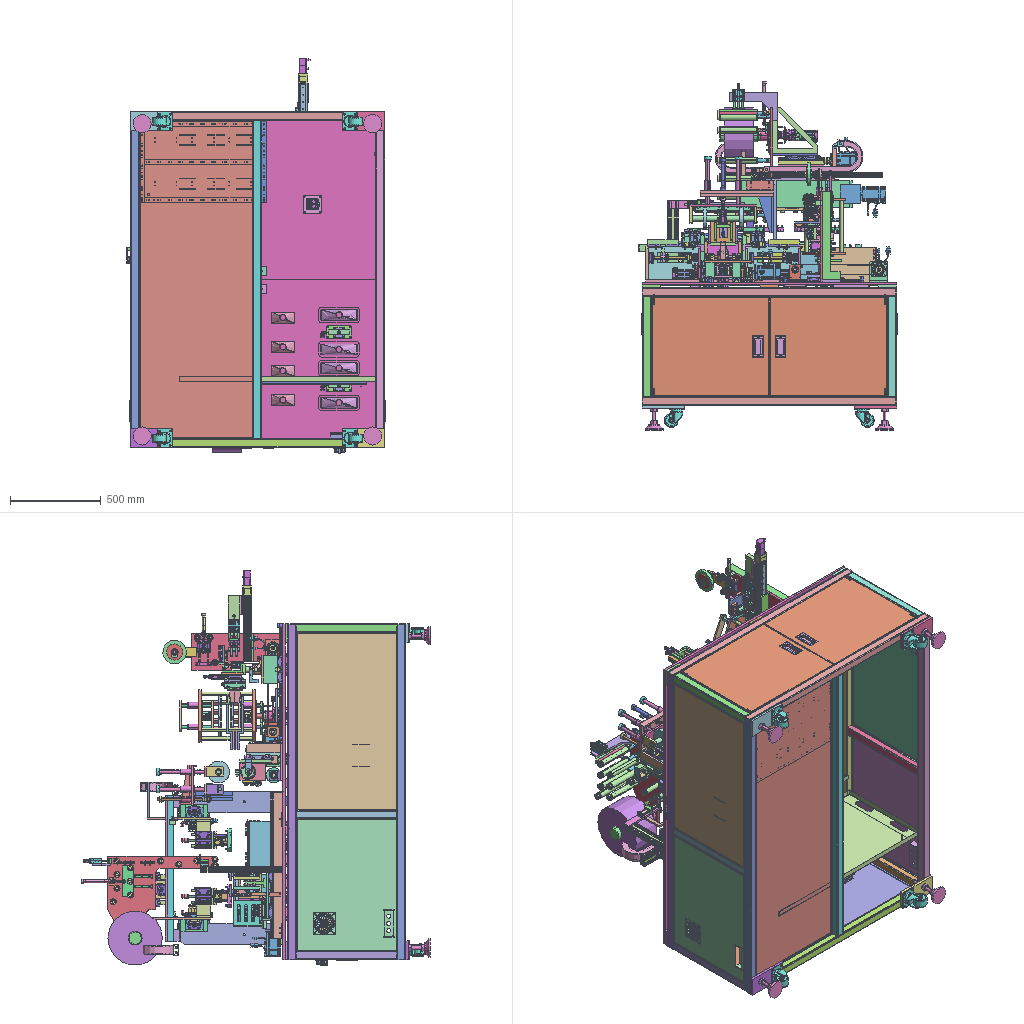Assembly | SolidWorks | 434 different items | 1246 placed | box 1425 x 1922 x 2174 mm
Parts list (item | name | quantity | parent item | size | volume | features), first 296 of 434 items:
1 | (subassembly) | x1 | - | - | 4869772 mm3 | features CompositeCurve 1
2 | (subassembly) | x3 | in 1 | 36 x 36 x 90 mm | 32561 mm3 | -
3 | (subassembly) | x2 | - | 274 x 476.237 x 327 mm | 5964747 mm3 | -
4 | (subassembly) | x2 | - | 273 x 282 x 303 mm | 1781179 mm3 | features InContextFeatHolder 4
5 | (subassembly) | x1 | - | - | - | -
6 | (subassembly) | x9 | in 5 | 34 x 292 x 34 mm | 157895 mm3 | -
7 | (subassembly) | x3 | in 5 | 34 x 267 x 34 mm | 150041 mm3 | -
8 | (subassembly) | x1 | in 5 | - | 5456068 mm3 | -
9 | (subassembly) | x1 | in 21 | - | 62540138 mm3 | -
10 | (subassembly) | x1 | - | 463.5 x 247.5 x 400.75 mm | 4348981 mm3 | features MirrorCompFeat 1
11 | (subassembly) | x1 | - | - | 21572641 mm3 | features CompositeCurve 32, InContextFeatHolder 3
12 | (subassembly) | x1 | - | 250 x 458 x 100.154 mm | 518648 mm3 | -
13 | (subassembly) | x1 | in 21 | 250.3 x 70.4 x 187 mm | 621495 mm3 | features AEMSimFeature 1
14 | (subassembly) | x1 | in 9 | - | 51712509 mm3 | -
15 | (subassembly) | x1 | - | - | 62540138 mm3 | features InContextFeatHolder 2
16 | (subassembly) | x10 | in 11, 21, 22 | 146.05 x 68.7 x 173.94 mm | 268514 mm3 | features ReferencePattern 3, AEMSimFeature 1, LocalLPattern 1
17 | (subassembly) | x1 | in 9 | 480 x 600 x 177.209 mm | 8711349 mm3 | -
18 | (subassembly) | x1 | - | - | 6443563 mm3 | features InContextFeatHolder 2, MirrorCompFeat 2
19 | (subassembly) | x2 | in 21 | 125.5 x 125.5 x 54.4 mm | 343156 mm3 | -
20 | (subassembly) | x1 | - | - | 6443563 mm3 | features InContextFeatHolder 8, MirrorCompFeat 2
21 | (subassembly) | x1 | - | - | - | features MirrorCompFeat 5, CompositeCurve 1
22 | (subassembly) | x1 | - | - | - | features InContextFeatHolder 8, CompositeCurve 2
23 | (subassembly) | x2 | in 22 | 148 x 205.5 x 218 mm | 1082273 mm3 | -
24 | (subassembly) | x1 | - | - | 10593540 mm3 | features CompositeCurve 3, InContextFeatHolder 2
25 | (subassembly) | x1 | - | - | - | features CompositeCurve 2, InContextFeatHolder 2
26 | (subassembly) | x1 | - | - | - | features CompositeCurve 3
27 | - | x3 | in 21 | 647 x 568 x 15 mm | 618702 mm3 | features ICE 5, FlatPattern 1, Helix 1, MirrorPattern 1, SMBaseFlange 1, SMMiteredFlange 1, SheetMetal 1, Sweep 1
28 | - | x1 | in 26 | 164 x 90 x 12 mm | 100831 mm3 | features Chamfer 1, Extrusion 1, Fillet 1
29 | - | x8 | in 26 | 40 x 30 x 12 mm | 14400 mm3 | features Extrusion 1
30 | - | x2 | in 26 | 180 x 150 x 10 mm | 230000 mm3 | features Extrusion 1, ICE 1, MirrorPattern 1
31 | - | x2 | in 26 | 180 x 150 x 6 mm | 138000 mm3 | features Extrusion 1, ICE 1, MirrorPattern 1
32 | - | x4 | in 26 | 12 x 12 x 75 mm | 8482 mm3 | features Extrusion 1
33 | - | x2 | in 26 | 60 x 90 x 14 mm | 56400 mm3 | features 3DProfileFeature 1, Chamfer 1, Extrusion 1, HoleWzd 1, ICE 1
34 | - | x1 | in 26 | 48 x 112.5 x 100 mm | 90182 mm3 | features Chamfer 1, Extrusion 1, ICE 1
35 | - | x1 | in 26 | 43 x 28 x 20 mm | 2700 mm3 | features FlatPattern 1, SMBaseFlange 1, SheetMetal 1
36 | - | x1 | in 26 | 95.861 x 40 x 61 mm | 9071 mm3 | features ICE 3, Extrusion 1
37 | - | x1 | in 1 | 17 x 58 x 27 mm | 21446 mm3 | features ICE 3, 3DProfileFeature 1, Extrusion 1, Fillet 1, HoleWzd 1
38 | - | x1 | in 21 | 647 x 568 x 78 mm | 637931 mm3 | features ICE 6, Cut 2, MirrorPattern 2, BossThin 1, Fillet 1, FlatPattern 1, Helix 1, SMBaseFlange 1, SMMiteredFlange 1, SheetMetal 1, Sweep 1, WeldmentFeature 1
39 | - | x1 | in 1 | 18 x 27 x 4 mm | 1881 mm3 | features Extrusion 1, ICE 1, LPattern 1, MirrorPattern 1
40 | - | x2 | in 1 | 10 x 27 x 4 mm | 1033 mm3 | features Extrusion 1, ICE 1, LPattern 1, MirrorPattern 1
41 | - | x2 | in 1 | 80 x 37 x 8 mm | 8818 mm3 | features ICE 4, 3DProfileFeature 1, Chamfer 1, Extrusion 1, Fillet 1, HoleWzd 1, MirrorPattern 1
42 | - | x2 | in 1 | 4 x 4 x 37 mm | 464.956 mm3 | features Extrusion 1
43 | - | x2 | in 1 | 9 x 9 x 28.5 mm | 1584 mm3 | features Extrusion 1
44 | - | x2 | in 1 | 4 x 4 x 47 mm | 590.619 mm3 | features Extrusion 1
45 | - | x1 | in 1 | 47 x 62 x 36 mm | 37251 mm3 | features ICE 6, 3DProfileFeature 2, HoleWzd 2, Extrusion 1, Fillet 1
46 | - | x1 | in 1 | 8 x 8 x 55 mm | 2765 mm3 | features Extrusion 1
47 | - | x2 | in 1 | 14 x 14 x 6 mm | 811.438 mm3 | features 3DProfileFeature 1, Chamfer 1, Extrusion 1, HoleWzd 1
48 | - | x1 | in 1 | 300 x 64 x 22.5 mm | 298859 mm3 | features ICE 4, Fillet 2, Extrusion 1, MirrorPattern 1
49 | - | x1 | in 21 | 1400 x 680 x 1850 mm | 13190709 mm3 | features WeldCornerFeat 8, Chamfer 4, HoleWzd 4, ICE 4, MirrorSolid 4, WeldMemberFeat 4, WeldmentFeature 1
50 | - | x1 | in 1 | 200 x 500 x 12 mm | 1093684 mm3 | features ICE 6, Fillet 2, Extrusion 1
51 | - | x1 | in 1 | 150 x 10 x 55 mm | 82500 mm3 | features Extrusion 1
52 | - | x1 | in 1 | 50 x 50 x 111 mm | 52677 mm3 | features ICE 3, Extrusion 1, RevCut 1
53 | - | x1 | in 1 | 46 x 40 x 46 mm | 14326 mm3 | features Revolution 1
54 | - | x1 | in 1 | 50 x 150 x 10 mm | 69893 mm3 | features Extrusion 1, ICE 1
55 | - | x1 | in 1 | 90 x 4 x 90 mm | 20564 mm3 | features Extrusion 1, ICE 1
56 | - | x1 | in 1 | 34 x 34 x 10 mm | 3614 mm3 | features Extrusion 1, HoleWzd 1
57 | - | x2 | in 1 | 87 x 22 x 12 mm | 17341 mm3 | features 3DProfileFeature 1, Extrusion 1, Fillet 1, HoleWzd 1, ICE 1, MirrorPattern 1
58 | - | x2 | in 1 | 8 x 8 x 140 mm | 7037 mm3 | features Extrusion 1
59 | - | x1 | in 1 | 25 x 72 x 50 mm | 71856 mm3 | features 3DProfileFeature 1, Chamfer 1, Extrusion 1, HoleWzd 1
60 | - | x1 | in 21 | 550 x 973 x 40 mm | 869590 mm3 | features ICE 2, BossThin 1, FlatPattern 1, SMBaseFlange 1, SMMiteredFlange 1, SheetMetal 1
61 | - | x1 | in 1 | 30 x 61 x 5 mm | 7526 mm3 | features Extrusion 1, Fillet 1
62 | - | x1 | in 1 | 53 x 14 x 63.5 mm | 9599 mm3 | features ICE 2, Extrusion 1
63 | - | x3 | in 2 | 12 x 12 x 90 mm | 9933 mm3 | features 3DProfileFeature 3, Extrusion 1, HoleWzd 1, ICE 1, LPattern 1, LibraryFeature 1, RefAxis 1, RevCut 1
64 | - | x4 | in 1, 2 | 27 x 27 x 50 mm | 13441 mm3 | features MirrorPattern 2, Extrusion 1, ICE 1, LPattern 1, RevCut 1
65 | - | x1 | in 1 | 90 x 4 x 90 mm | 23241 mm3 | features Extrusion 1, ICE 1
66 | - | x1 | in 1 | 45 x 57 x 10 mm | 13030 mm3 | features Extrusion 1, Fillet 1, ICE 1
67 | - | x1 | in 1 | 65 x 76 x 12 mm | 50562 mm3 | features ICE 2, 3DProfileFeature 1, Extrusion 1, HoleWzd 1
68 | - | x1 | in 1 | 80 x 60 x 12 mm | 45558 mm3 | features ICE 2, Extrusion 1, Fillet 1
69 | - | x1 | in 1 | 36 x 43 x 12 mm | 15546 mm3 | features ICE 3, Extrusion 1
70 | - | x2 | in 1 | 17.5 x 29 x 18 mm | 4245 mm3 | features ICE 3, Chamfer 1, Extrusion 1
71 | - | x2 | in 21 | 1400 x 925 x 14 mm | 18130000 mm3 | features Extrusion 1
72 | - | x1 | in 1 | 40 x 74.5 x 20 mm | 23378 mm3 | features ICE 2, Extrusion 1, LPattern 1
73 | - | x1 | in 1 | 44 x 35 x 13 mm | 17580 mm3 | features ICE 2, Extrusion 1, LPattern 1, MirrorPattern 1
74 | - | x1 | in 1 | 140 x 34 x 90 mm | 116009 mm3 | features ICE 2, Extrusion 1
75 | - | x2 | in 1, 10 | 43 x 22 x 0.4 mm | 344.471 mm3 | features Extrusion 1, ICE 1
76 | - | x1 | in 1 | 120 x 15 x 22 mm | 24706 mm3 | features ICE 4, Extrusion 1
77 | - | x1 | in 1 | 60 x 15 x 3 mm | 2658 mm3 | features 3DProfileFeature 1, Extrusion 1, HoleWzd 1
78 | - | x1 | in 1 | 55 x 100 x 12 mm | 58500 mm3 | features Extrusion 1, ICE 1
79 | - | x1 | in 1 | 200 x 100 x 12 mm | 240000 mm3 | features Extrusion 1
80 | - | x2 | in 1 | 98 x 488 x 12 mm | 292248 mm3 | features Chamfer 1, Extrusion 1, Fillet 1, ICE 1
81 | - | x8 | in 1, 2 | 36 x 36 x 8 mm | 3457 mm3 | features Extrusion 1, HoleWzd 1
82 | - | x1 | in 22 | 270 x 14 x 440 mm | 1620625 mm3 | features ICE 3, 3DProfileFeature 1, Extrusion 1, HoleWzd 1
83 | - | x6 | in 3 | 25 x 25 x 170 mm | 38250 mm3 | features Extrusion 1
84 | - | x2 | in 3 | 25 x 13 x 170 mm | 27963 mm3 | features 3DProfileFeature 1, Extrusion 1, HoleWzd 1
85 | - | x2 | in 3 | 130 x 12 x 180 mm | 252000 mm3 | features Extrusion 1
86 | - | x2 | in 3 | 210 x 12 x 260 mm | 560402 mm3 | features Chamfer 2, MirrorPattern 2, 3DProfileFeature 1, Extrusion 1, HoleWzd 1, ICE 1, LPattern 1
87 | - | x4 | in 3 | 23 x 23 x 180 mm | 21634 mm3 | features ICE 2, Extrusion 1, MirrorPattern 1
88 | - | x4 | in 3 | 160 x 25 x 7 mm | 28000 mm3 | features Extrusion 1
89 | - | x2 | in 3 | 140 x 25 x 5 mm | 17500 mm3 | features Extrusion 1
90 | - | x4 | in 3 | 16 x 22.5 x 190 mm | 52215 mm3 | features Chamfer 2, Extrusion 1, ICE 1
91 | - | x2 | in 3 | 18 x 16 x 190 mm | 52178 mm3 | features Chamfer 1, Extrusion 1, ICE 1
92 | - | x2 | in 3 | 135 x 70 x 8 mm | 55222 mm3 | features ICE 3, Chamfer 1, Extrusion 1
93 | - | x1 | in 22 | 55 x 44 x 35 mm | 54034 mm3 | features HoleWzd 2, 3DProfileFeature 1, Extrusion 1
94 | - | x4 | in 3 | 16 x 16 x 280 mm | 56297 mm3 | features Extrusion 1
95 | - | x2 | in 3 | 60 x 10 x 120 mm | 62330 mm3 | features ICE 2, Chamfer 1, Extrusion 1
96 | - | x8 | in 3 | 12 x 12 x 40 mm | 4146 mm3 | features 3DProfileFeature 1, Extrusion 1, HoleWzd 1, MirrorPattern 1
97 | - | x2 | in 3 | 25 x 10 x 120 mm | 26926 mm3 | features ICE 2, Extrusion 1
98 | - | x2 | in 3 | 19 x 18 x 7 mm | 1848 mm3 | features Extrusion 1
99 | - | x8 | in 3 | 24 x 24 x 10 mm | 2386 mm3 | features Extrusion 1
100 | - | x4 | in 3 | 260 x 15 x 5 mm | 19460 mm3 | features Chamfer 1, Extrusion 1
101 | - | x2 | in 3 | 41.958 x 24 x 12 mm | 3447 mm3 | features Extrusion 1, ICE 1
102 | - | x2 | in 3 | 260 x 20 x 20 mm | 43442 mm3 | features WeldMemberFeat 1, WeldmentFeature 1
103 | - | x2 | in 3 | 309 x 192.237 x 274 mm | 268790 mm3 | features EdgeFlange 2, FlatPattern 1, ICE 1, MirrorPattern 1, SMBaseFlange 1, SheetMetal 1
104 | - | x2 | in 22 | 25 x 53 x 800 mm | 1009600 mm3 | features Extrusion 1
105 | - | x2 | in 3 | 170 x 14 x 10 mm | 23403 mm3 | features 3DProfileFeature 1, Extrusion 1, HoleWzd 1, MirrorPattern 1
106 | - | x2 | in 3 | 248 x 185 x 6 mm | 275280 mm3 | features Extrusion 1
107 | - | x4 | in 3 | 224 x 84 x 115 mm | 101490 mm3 | features ICE 2, Blend 1, Extrusion 1, Shell 1
108 | - | x8 | in 3 | 40 x 30 x 12 mm | 6087 mm3 | features Extrusion 1, ICE 1, LPattern 1, MirrorPattern 1
109 | - | x8 | in 3 | 30 x 65 x 3 mm | 4682 mm3 | features Extrusion 1, ICE 1, MirrorPattern 1
110 | - | x4 | in 3 | 21 x 25 x 5 mm | 1150 mm3 | features Extrusion 1
111 | - | x2 | in 4 | 170 x 10 x 210 mm | 352545 mm3 | features MirrorPattern 2, Chamfer 1, Cut 1, Extrusion 1, ICE 1
112 | - | x8 | in 4 | 46 x 30 x 10 mm | 11809 mm3 | features 3DProfileFeature 1, Extrusion 1, HoleWzd 1, ICE 1, MirrorPattern 1
113 | - | x2 | in 4 | 135 x 180 x 8 mm | 157363 mm3 | features ICE 2, Chamfer 1, Extrusion 1
114 | - | x6 | in 4 | 80 x 42 x 10 mm | 29577 mm3 | features ICE 2, Chamfer 1, Extrusion 1, MirrorPattern 1
115 | - | x1 | in 22 | 48 x 93 x 100 mm | 106256 mm3 | features Chamfer 1, Extrusion 1
116 | - | x2 | in 4 | 58 x 62 x 10 mm | 30557 mm3 | features ICE 2, Chamfer 1, Extrusion 1, MirrorPattern 1
117 | - | x8 | in 4 | 20 x 20 x 150 mm | 47124 mm3 | features Extrusion 1
118 | - | x2 | in 4 | 245 x 10 x 210 mm | 367454 mm3 | features MirrorPattern 3, 3DProfileFeature 1, Chamfer 1, Cut 1, Extrusion 1, HoleWzd 1, ICE 1
119 | - | x4 | in 4 | 154 x 84 x 100 mm | 51797 mm3 | features ICE 2, Blend 1, Extrusion 1, Shell 1
120 | - | x2 | in 4 | 273 x 181.2 x 303 mm | 301154 mm3 | features Chamfer 1, ExtruThin 1, ICE 1
121 | - | x2 | in 11 | 600 x 150 x 14 mm | 1207472 mm3 | features ICE 3, Extrusion 1, Fillet 1
122 | - | x4 | in 11 | 25 x 33 x 600 mm | 457200 mm3 | features Extrusion 1
123 | - | x4 | in 11 | 14 x 550 x 115 mm | 786870 mm3 | features ICE 2, Chamfer 1, Extrusion 1
124 | - | x2 | in 11 | 300 x 12 x 115 mm | 414000 mm3 | features Extrusion 1
125 | - | x8 | in 11 | 74 x 74 x 20 mm | 33836 mm3 | features 3DProfileFeature 2, Chamfer 2, HoleWzd 2, Extrusion 1, Fillet 1
126 | - | x1 | in 22 | 25 x 90 x 24.5 mm | 55125 mm3 | features Extrusion 1
127 | - | x2 | in 11 | 272 x 25 x 25 mm | 133518 mm3 | features Extrusion 1
128 | - | x2 | in 11 | 300 x 180 x 12 mm | 604823 mm3 | features ICE 3, Extrusion 1, MirrorPattern 1
129 | - | x2 | in 11 | 112 x 95 x 100 mm | 206190 mm3 | features ICE 2, Chamfer 1, Extrusion 1
130 | - | x4 | in 11 | 34 x 80 x 162 mm | 152640 mm3 | features Extrusion 1, ICE 1, MirrorPattern 1
131 | - | x2 | in 11 | 145 x 125 x 20 mm | 332455 mm3 | features ICE 4, Chamfer 1, Extrusion 1
132 | - | x2 | in 11 | 91 x 80 x 38 mm | 128587 mm3 | features Extrusion 1, Fillet 1, ICE 1
133 | - | x2 | in 11 | 145 x 125 x 20 mm | 303441 mm3 | features ICE 6, Chamfer 1, Extrusion 1
134 | - | x4 | in 11 | 38 x 80 x 24 mm | 29184 mm3 | features Extrusion 1, ICE 1
135 | - | x1 | in 11 | 55 x 47 x 35 mm | 59809 mm3 | features HoleWzd 2, 3DProfileFeature 1, Extrusion 1
136 | - | x2 | in 11 | 18 x 8 x 30 mm | 2093 mm3 | features 3DProfileFeature 1, Extrusion 1, HoleWzd 1, ICE 1, MirrorPattern 1
137 | - | x1 | in 17 | 440 x 300 x 58 mm | 6630448 mm3 | features ICE 7, Fillet 2, Chamfer 1, Extrusion 1, HoleWzd 1, LPattern 1
138 | - | x1 | in 22 | 20 x 90 x 24.5 mm | 44100 mm3 | features Extrusion 1
139 | - | x6 | in 11 | 25 x 70 x 14 mm | 24500 mm3 | features Extrusion 1
140 | - | x2 | in 11 | 600 x 30 x 60 mm | 465086 mm3 | features WeldMemberFeat 1, WeldmentFeature 1
141 | - | x2 | in 11 | 170 x 214 x 10 mm | 60475 mm3 | features ICE 2, Chamfer 1, Extrusion 1, Fillet 1
142 | - | x2 | in 11 | 20 x 195 x 10 mm | 39000 mm3 | features Extrusion 1
143 | - | x2 | in 11 | 300 x 73 x 62 mm | 429281 mm3 | features ICE 6, Extrusion 1, Fillet 1
144 | - | x1 | in 5 | 600 x 515 x 14 mm | 1803753 mm3 | features ICE 11, Chamfer 4, Fillet 3, Cut 1, Extrusion 1
145 | - | x1 | in 5 | 30 x 30 x 17 mm | 3335 mm3 | features Extrusion 1
146 | - | x1 | in 5 | 65 x 68 x 120 mm | 106942 mm3 | features ICE 5, MirrorPattern 3, Chamfer 1, WeldMemberFeat 1, WeldmentFeature 1
147 | - | x1 | in 5 | 12 x 45 x 10 mm | 4126 mm3 | features 3DProfileFeature 1, Chamfer 1, Extrusion 1, HoleWzd 1, ICE 1, MirrorPattern 1
148 | - | x13 | in 6, 7, 10 | 210 x 34 x 34 mm | 85831 mm3 | features Revolution 1
149 | - | x1 | in 22 | 180 x 182 x 14 mm | 257706 mm3 | features ICE 5, Extrusion 1, Fillet 1
150 | - | x9 | in 6 | 20 x 20 x 275 mm | 57016 mm3 | features ICE 2, 3DProfileFeature 1, Extrusion 1, HoleWzd 1
151 | - | x12 | in 6, 7 | 33 x 33 x 14 mm | 9032 mm3 | features ICE 2, Chamfer 1, Extrusion 1
152 | - | x1 | in 5 | 170 x 60 x 12 mm | 111868 mm3 | features ICE 2, 3DProfileFeature 1, Extrusion 1, HoleWzd 1
153 | - | x1 | in 5 | 23 x 42 x 40 mm | 17172 mm3 | features Extrusion 1, ICE 1
154 | - | x1 | in 5 | 269 x 155 x 12 mm | 212510 mm3 | features Cut 1, Extrusion 1
155 | - | x1 | in 5 | 210 x 28 x 14 mm | 79716 mm3 | features Extrusion 1, ICE 1
156 | - | x1 | in 5 | 28 x 17 x 210 mm | 85260 mm3 | features Extrusion 1
157 | - | x1 | in 8 | 215 x 14 x 250 mm | 709650 mm3 | features ICE 2, Chamfer 1, Extrusion 1, Fillet 1
158 | - | x2 | in 8 | 250 x 245 x 12 mm | 232707 mm3 | features Extrusion 1
159 | - | x2 | in 8 | 25 x 28.5 x 250 mm | 162375 mm3 | features Extrusion 1
160 | - | x1 | in 22 | 55 x 75.5 x 30 mm | 98100 mm3 | features HoleWzd 2, 3DProfileFeature 1, Extrusion 1
161 | - | x1 | in 8 | 55 x 44 x 35 mm | 59279 mm3 | features HoleWzd 2, 3DProfileFeature 1, Extrusion 1
162 | - | x1 | in 8 | 250 x 800 x 14 mm | 1757091 mm3 | features ICE 2, Extrusion 1, Fillet 1
163 | - | x2 | in 8 | 800 x 14 x 30 mm | 336000 mm3 | features Extrusion 1
164 | - | x1 | in 8 | 45 x 101 x 100 mm | 97106 mm3 | features 3DProfileFeature 1, Chamfer 1, Extrusion 1, HoleWzd 1, ICE 1
165 | - | x3 | in 7 | 20 x 20 x 250 mm | 49162 mm3 | features ICE 2, 3DProfileFeature 1, Extrusion 1, HoleWzd 1
166 | - | x1 | in 14 | 1840 x 1100 x 1390 mm | 30476002 mm3 | features ICE 16, WeldCornerFeat 14, HoleWzd 8, WeldMemberFeat 7, MirrorPattern 3, Fillet 2, 3DProfileFeature 1, Cut 1, WeldmentFeature 1
167 | - | x1 | in 10 | 403 x 225.5 x 32 mm | 1138849 mm3 | features ICE 3, MoveFace 2, Extrusion 1
168 | - | x1 | in 10 | 240 x 25 x 12 mm | 71196 mm3 | features Extrusion 1, ICE 1
169 | - | x2 | in 10 | 23 x 31 x 10 mm | 4928 mm3 | features 3DProfileFeature 3, HoleWzd 3, ICE 2, Chamfer 1, Extrusion 1
170 | - | x2 | in 10 | 22 x 22 x 5 mm | 831.54 mm3 | features Extrusion 1
171 | - | x1 | in 22 | 60 x 180 x 14 mm | 46123 mm3 | features Extrusion 1, Fillet 1, ICE 1
172 | - | x2 | in 10 | 55 x 35 x 4 mm | 5554 mm3 | features Chamfer 1, Extrusion 1, ICE 1, MirrorPattern 1
173 | - | x1 | in 10 | 365 x 55 x 12 mm | 237663 mm3 | features ICE 2, Extrusion 1
174 | - | x2 | in 10 | 55 x 80 x 12 mm | 48578 mm3 | features ICE 3, 3DProfileFeature 1, Chamfer 1, Extrusion 1, HoleWzd 1
175 | - | x1 | in 10 | 20 x 14 x 370 mm | 68901 mm3 | features ICE 2, Extrusion 1
176 | - | x1 | in 10 | 32 x 30 x 63 mm | 43546 mm3 | features ICE 2, 3DProfileFeature 1, Extrusion 1, HoleWzd 1
177 | - | x2 | in 10 | 35 x 9 x 3 mm | 849.574 mm3 | features Extrusion 1
178 | - | x1 | in 10 | 50 x 12 x 3 mm | 1705 mm3 | features Extrusion 1
179 | - | x1 | in 10 | 365 x 55 x 12 mm | 237663 mm3 | features ICE 2, Extrusion 1
180 | - | x2 | in 10 | 55 x 94.5 x 12 mm | 49827 mm3 | features ICE 4, Chamfer 1, Extrusion 1
181 | - | x1 | in 10 | 30 x 30 x 361 mm | 247322 mm3 | features Extrusion 1, ICE 1, MirrorPattern 1
182 | - | x1 | in 22 | 150 x 14 x 200 mm | 400905 mm3 | features ICE 2, 3DProfileFeature 1, Extrusion 1, HoleWzd 1
183 | - | x1 | - | 217.5 x 60 x 150 mm | 433717 mm3 | features ICE 2, Chamfer 1, Extrusion 1, Fillet 1, MirrorPattern 1
184 | - | x1 | - | 217.5 x 90 x 50 mm | 220780 mm3 | features Chamfer 1, Extrusion 1, ICE 1
185 | - | x1 | in 12 | 30 x 450 x 60 mm | 348814 mm3 | features WeldMemberFeat 1, WeldmentFeature 1
186 | - | x1 | in 12 | 250 x 40 x 10 mm | 95200 mm3 | features Extrusion 1, ICE 1
187 | - | x2 | in 12 | 40 x 12 x 23 mm | 9230 mm3 | features ICE 5, Extrusion 1
188 | - | x1 | in 12 | 12 x 12 x 157 mm | 15432 mm3 | features ICE 2, Extrusion 1
189 | - | x2 | in 12 | 8 x 8 x 144 mm | 7238 mm3 | features Extrusion 1
190 | - | x1 | in 12 | 40 x 20 x 25 mm | 16355 mm3 | features ICE 5, 3DProfileFeature 1, Extrusion 1, HoleWzd 1
191 | - | x1 | in 12 | 70 x 55 x 4 mm | 7768 mm3 | features Fillet 2, ICE 2, Extrusion 1
192 | - | x7 | in 5, 22, 24, 25, 26 | - | 141786 mm3 | features BaseBody 32
193 | - | x1 | in 22 | 200 x 14 x 165 mm | 371300 mm3 | features Extrusion 1, Fillet 1, ICE 1
194 | - | x20 | in 16 | 22 x 64 x 22 mm | 21333 mm3 | features BaseBody 1
195 | - | x38 | in 3, 5, 11, 22, 24, 25, 26 | 13.7 x 28.4 x 26 mm | 1939 mm3 | features BaseBody 1
196 | - | x2 | in 13 | 21 x 8.5 x 8.5 mm | 552.853 mm3 | features BaseBody 1
197 | - | x1 | in 13 | 68.8 x 64 x 160 mm | 171745 mm3 | features BaseBody 2
198 | - | x1 | in 13 | 68.8 x 64 x 171.6 mm | 182520 mm3 | features BaseBody 1
199 | - | x2 | in 13 | 33 x 49.1 x 93 mm | 35639 mm3 | features BaseBody 1
200 | - | x2 | in 13 | 11.9 x 33 x 25 mm | 6485 mm3 | features BaseBody 1
201 | - | x1 | in 13 | 68.8 x 68.4 x 103.9 mm | 177481 mm3 | features BaseBody 5
202 | - | x1 | in 24 | 60 x 95 x 137 mm | 414579 mm3 | features BaseBody 8
203 | - | x1 | in 21 | 450 x 700 x 6 mm | 1886062 mm3 | features HoleWzd 2, Cut 1, Extrusion 1
204 | - | x3 | in 22 | 135 x 150 x 14 mm | 55621 mm3 | features Extrusion 1, Fillet 1, ICE 1
205 | - | x1 | in 14 | 150 x 3 x 150 mm | 65828 mm3 | features Extrusion 1, Fillet 1, HoleWzd 1, ICE 1
206 | - | x1 | in 17 | 480 x 600 x 153 mm | 803618 mm3 | features ICE 7, EdgeFlange 3, Cut 1, FlatPattern 1, SMBaseFlange 1, SheetMetal 1
207 | - | x1 | in 9 | 480 x 195.932 x 160.122 mm | 336686 mm3 | features EdgeFlange 8, ICE 2, Fillet 1, FlatPattern 1, SMBaseFlange 1, SheetMetal 1
208 | - | x6 | in 9 | 49.2 x 40 x 8 mm | 11464 mm3 | features HoleWzd 2, ICE 2, Chamfer 1, Extrusion 1
209 | - | x2 | in 14 | 718 x 1016 x 28.7 mm | 4599989 mm3 | features MoveCopyBody 3, Stock 3, ICE 2, HoleWzd 1, WeldMemberFeat 1, WeldmentFeature 1
210 | - | x2 | in 14 | 588 x 1016 x 28.7 mm | 3776300 mm3 | features MoveCopyBody 3, Stock 3, ICE 2, HoleWzd 1, WeldMemberFeat 1, WeldmentFeature 1
211 | - | x2 | in 14 | 479 x 716 x 28.7 mm | 2209048 mm3 | features MoveCopyBody 3, Stock 3, ICE 2, HoleWzd 1, WeldMemberFeat 1, WeldmentFeature 1
212 | - | x10 | in 16 | 60 x 26.5 x 140 mm | 117754 mm3 | features 3DProfileFeature 3, HoleWzd 3, Cut 1, Extrusion 1, LPattern 1
213 | - | x40 | in 16 | 15.02 x 42.2 x 146.05 mm | 33782 mm3 | features Boss 25, Cut 6, RevCut 5, Revolution 2, Extrusion 1, ICE 1
214 | - | x2 | in 4 | 41.439 x 18 x 38.614 mm | 6724 mm3 | features Chamfer 1, Extrusion 1, Sweep 1
215 | - | x1 | in 22 | 93 x 62 x 40 mm | 39399 mm3 | features ICE 5, 3DProfileFeature 1, Extrusion 1, Fillet 1, HoleWzd 1
216 | - | x2 | in 11 | 24 x 27.713 x 90.43 mm | 14815 mm3 | features ICE 3, Chamfer 2, Extrusion 1, MirrorPattern 1, Sweep 1
217 | - | x4 | in 11 | 53.2 x 29.75 x 23 mm | 14418 mm3 | features ICE 8, Revolution 1
218 | - | x1 | in 17 | 212.35 x 146.35 x 53.56 mm | 1066070 mm3 | features ICE 16, Fillet 5, MirrorPattern 2, Extrusion 1, HoleWzd 1
219 | - | x6 | in 9 | 49.2 x 17.45 x 45.25 mm | 22167 mm3 | features ICE 16, Chamfer 3, Fillet 3, Extrusion 1
220 | - | x1 | in 9 | 330 x 19.5 x 178 mm | 879010 mm3 | features ICE 7, Fillet 4, LPattern 2, Extrusion 1
221 | - | x2 | in 1, 5 | 142 x 64.5 x 30.5 mm | 123936 mm3 | features BaseBody 5, MoveFace 1
222 | - | x2 | in 3 | 57 x 57 x 276 mm | 233690 mm3 | features ICE 6, Extrusion 1, Fillet 1, MoveFace 1
223 | - | x5 | in 11, 22, 24 | 45 x 53 x 34 mm | 37006 mm3 | features BaseBody 1
224 | - | x2 | in 3 | 130 x 150 x 180 mm | 3150000 mm3 | features Extrusion 1
225 | - | x3 | in 25 | 9 x 6 x 50 mm | 1608 mm3 | features Extrusion 1
226 | - | x1 | in 22 | 60 x 180 x 14 mm | 45584 mm3 | features Cut 1, Extrusion 1, Fillet 1, ICE 1
227 | - | x18 | in 5, 11, 22, 24, 25, 26 | 9 x 6 x 75 mm | 2412 mm3 | features Extrusion 1
228 | - | x1 | in 22 | 9 x 6 x 75 mm | 2412 mm3 | features Extrusion 1
229 | - | x1 | in 10 | 15 x 15 x 240 mm | 42412 mm3 | features Extrusion 1
230 | - | x2 | in 10 | 16 x 16 x 250 mm | 50265 mm3 | features Extrusion 1
231 | - | x4 | in 10 | 20 x 20 x 265 mm | 83252 mm3 | features Extrusion 1
232 | - | x4 | in 11 | 24.892 x 60.174 x 63.5 mm | 25312 mm3 | features BaseBody 8
233 | - | x2 | in 1 | 45 x 32 x 32 mm | 7447 mm3 | features BaseBody 1
234 | - | x3 | in 10 | 120 x 120 x 20 mm | 212058 mm3 | features Extrusion 1
235 | - | x1 | in 17 | 30 x 78.5 x 40 mm | 52539 mm3 | features Boss 3, Revolution 2, Cut 1, Fillet 1
236 | - | x4 | in 25, 26 | 35 x 6 x 42 mm | 6903 mm3 | features BaseBody 1
237 | - | x2 | in 23 | 46 x 119 x 100 mm | 191222 mm3 | features ICE 2, MirrorPattern 2, Extrusion 1
238 | - | x2 | in 1 | 92 x 46 x 17 mm | 51092 mm3 | features BaseBody 2, MoveFace 1
239 | - | x8 | in 4 | 68 x 42 x 17 mm | 36294 mm3 | features BaseBody 2, MoveFace 1
240 | - | x4 | in 11 | 176.5 x 93 x 42 mm | 329147 mm3 | features BaseBody 3, MoveFace 1
241 | - | x6 | in 8, 11, 22, 25, 26 | 104.241 x 167.272 x 173.3 mm | 816769 mm3 | features BaseBody 1
242 | - | x4 | in 3 | 17.5 x 17.5 x 55 mm | 1534 mm3 | features BaseBody 2, MoveFace 2, CoordSys 1
243 | - | x2 | in 25, 26 | 515 x 55 x 25 mm | 54325 mm3 | features ExtruThin 1
244 | - | x3 | in 22, 24 | 22 x 48 x 48 mm | 28934 mm3 | features BaseBody 1
245 | - | x1 | in 24 | 32 x 55 x 55 mm | 52760 mm3 | features BaseBody 1
246 | - | x2 | in 24 | 31 x 83 x 83 mm | 73230 mm3 | features MoveFace 2, BaseBody 1, ICE 1
247 | - | x2 | in 24 | 31 x 83 x 83 mm | 94794 mm3 | features MoveFace 2, BaseBody 1, ICE 1
248 | - | x1 | in 21 | 550 x 723 x 40 mm | 641172 mm3 | features ICE 3, BossThin 1, FlatPattern 1, SMBaseFlange 1, SMMiteredFlange 1, SheetMetal 1
249 | - | x2 | in 23 | 60 x 140 x 14 mm | 109393 mm3 | features ICE 2, Cut 1, Extrusion 1, Fillet 1, HoleWzd 1
250 | - | x3 | in 22, 24 | 34 x 45 x 45 mm | 28395 mm3 | features BaseBody 1
251 | - | x2 | in 5 | 32 x 48 x 48 mm | 32144 mm3 | features BaseBody 1
252 | - | x2 | in 25, 26 | 32 x 55 x 55 mm | 48801 mm3 | features BaseBody 1, ICE 1
253 | - | x3 | in 24, 25, 26 | 44 x 55 x 55 mm | 58825 mm3 | features BaseBody 1
254 | - | x1 | in 17 | 30 x 78.5 x 40 mm | 52539 mm3 | features Boss 3, Revolution 2, Cut 1, Fillet 1
255 | - | x2 | in 10 | 35 x 35 x 15 mm | 11416 mm3 | features Extrusion 1
256 | - | x4 | in 10 | 40 x 40 x 15 mm | 14137 mm3 | features Extrusion 1
257 | - | x7 | in 8, 11, 22, 24 | 38 x 43 x 60 mm | 55106 mm3 | features BaseBody 9
258 | - | x3 | in 8, 25, 26 | 10 x 56 x 10 mm | 1814 mm3 | features BaseBody 1, MoveFace 1
259 | - | x1 | in 10 | 214 x 25 x 22 mm | 42451 mm3 | features BaseBody 4, MoveFace 2
260 | - | x2 | in 23 | 45 x 102 x 18 mm | 31894 mm3 | features 3DProfileFeature 1, Extrusion 1, Fillet 1, HoleWzd 1, ICE 1, MirrorPattern 1
261 | - | x1 | in 5 | 318 x 25 x 22 mm | 45425 mm3 | -
262 | - | x4 | in 23 | 158 x 25 x 22 mm | 25129 mm3 | features BaseBody 4, MoveFace 2
263 | - | x1 | in 1 | 148 x 25 x 22 mm | 28789 mm3 | features BaseBody 4, MoveFace 2
264 | - | x2 | in 10 | 216 x 33 x 29 mm | 70074 mm3 | features BaseBody 4, MoveFace 2
265 | - | x20 | in 16 | 10 x 14.097 x 14.097 mm | 1197 mm3 | features Chamfer 1, Cut 1, Revolution 1
266 | - | x3 | in 24 | 18 x 45 x 18 mm | 5618 mm3 | features BaseBody 1, MoveFace 1
267 | - | x5 | in 1, 5, 23 | 10 x 43.5 x 10 mm | 1326 mm3 | features BaseBody 1, MoveFace 1
268 | - | x1 | in 17 | 30 x 78.5 x 40 mm | 52539 mm3 | features Boss 3, Revolution 2, Cut 1, Fillet 1
269 | - | x3 | in 24 | 17 x 8 x 19.63 mm | 1532 mm3 | features BaseBody 1
270 | - | x1 | in 9 | 100 x 455.5 x 100 mm | 698561 mm3 | features ICE 17, Fillet 6, BossThin 1, Chamfer 1, CirPattern 1, Extrusion 1, RefAxis 1, RevCut 1
271 | - | x4 | in 23 | 60 x 60 x 12 mm | 30812 mm3 | features 3DProfileFeature 1, Extrusion 1, HoleWzd 1, ICE 1, LPattern 1, MirrorPattern 1
272 | - | x4 | in 22 | 64.1 x 19.5 x 34 mm | 30819 mm3 | features BaseBody 1
273 | - | x35 | in 1, 8, 11, 22, 24, 25, 26 | 83.53 x 22 x 42 mm | 51004 mm3 | features BaseBody 1
274 | - | x10 | in 5, 23 | 42.1 x 12 x 32 mm | 11943 mm3 | features BaseBody 1
275 | - | x4 | in 3 | 14 x 20 x 7 mm | 1562 mm3 | features ICE 2, Extrusion 1, Fillet 1, MirrorPattern 1
276 | - | x1 | - | 120 x 60 x 15 mm | 20369 mm3 | features Boss 2, Cut 1, Extrusion 1, Fillet 1, Shell 1
277 | - | x1 | in 24 | 51 x 53 x 31 mm | 42368 mm3 | features BaseBody 2
278 | - | x4 | in 24 | 55 x 61 x 35 mm | 59445 mm3 | features BaseBody 2
279 | - | x2 | in 5, 26 | 86 x 98 x 98 mm | 237483 mm3 | features BaseBody 5
280 | - | x2 | in 1 | 11 x 11 x 12 mm | 96.988 mm3 | features Helix 1, ICE 1, Sweep 1
281 | - | x1 | in 1 | 30 x 30 x 40 mm | 1368 mm3 | features Helix 1, ICE 1, Sweep 1
282 | - | x4 | in 23 | 30 x 95 x 11 mm | 13468 mm3 | features ICE 2, Extrusion 1, Fillet 1
283 | - | x20 | in 16 | 15.2 x 36.1 x 31.083 mm | 5569 mm3 | features BaseBody 1
284 | - | x1 | in 17 | 40 x 67.009 x 40 mm | 39506 mm3 | features Cut 3, Fillet 3, Boss 2, Revolution 1
285 | - | x1 | in 24 | 32 x 45 x 45 mm | 40105 mm3 | features BaseBody 4
286 | - | x4 | in 3 | 20 x 36 x 106 mm | 20303 mm3 | features BaseBody 1
287 | - | x2 | in 11 | 572.2 x 175 x 53 mm | 617417 mm3 | features BaseBody 3
288 | - | x1 | in 25 | 480.2 x 175 x 53 mm | 549939 mm3 | features BaseBody 3
289 | - | x1 | in 13 | 28.083 x 33.4 x 14 mm | 4394 mm3 | features BaseBody 1
290 | - | x1 | in 25 | 47 x 11 x 47 mm | 10056 mm3 | features BaseBody 1
291 | - | x7 | in 8, 11, 22, 24 | 20 x 43 x 60 mm | 35576 mm3 | features BaseBody 3
292 | - | x1 | in 5 | 300 x 300 x 160 mm | 10583900 mm3 | features Extrusion 1
293 | - | x2 | in 23 | 60 x 140 x 14 mm | 109393 mm3 | features ICE 2, Cut 1, Extrusion 1, Fillet 1, HoleWzd 1
294 | - | x1 | in 25 | 165 x 67.1 x 26.6 mm | 85115 mm3 | features BaseBody 9, MoveFace 3
295 | - | x1 | in 10 | 336 x 61 x 36 mm | 312285 mm3 | features BaseBody 4, MoveFace 1
296 | - | x4 | in 21 | 105 x 104 x 107.5 mm | 293798 mm3 | features ICE 10, Fillet 8, Chamfer 1, Extrusion 1
Mates (type | each side: item.copy, entity, surface, feature), first 256 of 2087 lines:
In the top assembly
Coincident | 71.1 face plane  Boss - Extrude 1 | 104.1 face plane  Boss - Extrude 1
Parallel | 71.1 face plane  Boss - Extrude 1 | 104.1 edge
Coincident | 71.2 face plane  Boss - Extrude 1 | 374.1 face plane  Boss - Extrude 1
Width | 104.2 face plane  Boss - Extrude 1 | 104.1 face plane  Boss - Extrude 1 | 374.1 face plane  Boss - Extrude 1 | 374.1 face plane  Boss - Extrude 1
Coincident | 71.2 face plane  Boss - Extrude 1 | 322.1 face plane  Boss - Extrude 1
Width | 104.2 face plane  Boss - Extrude 1 | 104.1 face plane  Boss - Extrude 1 | 390.1 face plane  Boss - Extrude 1 | 390.1 face plane  Boss - Extrude 1
DistanceDim | 407.1 face plane  Boss - Extrude 1 | 374.1 face plane  Boss - Extrude 1
DistanceDim | 374.1 face plane  Boss - Extrude 1 | 104.2 face plane  Boss - Extrude 1
DistanceDim | 374.1 face plane  Boss - Extrude 1 | 71.2 face plane  Boss - Extrude 1
Coincident | 71.2 face plane  Boss - Extrude 1 | 322.2 face plane  Boss - Extrude 1
Parallel | 71.2 face plane  Boss - Extrude 1 | 322.3 face plane  Boss - Extrude 1
Coincident | 71.2 face plane  Boss - Extrude 1 | 79.1 face plane  Boss - Extrude 1
Coincident | 71.1 face plane  Boss - Extrude 1 | 103.1 face plane  Edge - Flange 2
Parallel | 71.1 face plane  Boss - Extrude 1 | 103.1 face plane  Base - Flange 1
Coincident | 71.1 face plane  Boss - Extrude 1 | 103.2 face plane  Edge - Flange 2
Coincident | 103.1 face plane  Base - Flange 1 | 103.2 face plane  Base - Flange 1
Coincident | 71.1 face plane  Boss - Extrude 1 | 120.1 face plane  Boss - Extrude 1
Width | 103.2 face plane  Base - Flange 1 | 103.2 face plane  Base - Flange 1 | 120.1 face plane  Extrude - Thin-Wall 1 | 120.1 face plane  Extrude - Thin-Wall 1
Coincident | 71.1 face plane  Boss - Extrude 1 | 120.2 face plane  Boss - Extrude 1
Coincident | 120.1 face plane  Extrude - Thin-Wall 1 | 120.2 face plane  Extrude - Thin-Wall 1
Width | 103.1 face plane  Base - Flange 1 | 103.1 face plane  Base - Flange 1 | 120.2 face plane  Extrude - Thin-Wall 1 | 120.2 face plane  Extrude - Thin-Wall 1
DistanceDim | 103.1 face plane  Base - Flange 1 | 103.2 face plane  Base - Flange 1
DistanceDim | 241.1 face plane  Import 1 | 71.1 face plane  Boss - Extrude 1
Coincident | 71.1 face plane  Boss - Extrude 1 | 124.1 face plane  Boss - Extrude 1
Parallel | 71.1 face plane  Boss - Extrude 1 | 124.1 face plane  Boss - Extrude 1
Parallel | 71.1 face plane  Boss - Extrude 1 | 162.1 face plane  Boss - Extrude 1
Parallel | 71.1 face plane  Boss - Extrude 1 | 163.1 face plane  Boss - Extrude 1
DistanceDim | 123.1 face plane  Boss - Extrude 1 | 104.2 face plane  Boss - Extrude 1
Coincident | assembly face | 162.1 face plane  Boss - Extrude 1 | 2 times
Coincident | assembly face | 163.1 face plane  Boss - Extrude 1
Coincident | 143.1 face plane  Boss - Extrude 2 | 163.1 face plane  Boss - Extrude 1
Coincident | 143.1 face plane  Boss - Extrude 3 | 162.1 face plane  Boss - Extrude 1
Coincident | 143.1 face plane  Boss - Extrude 1 | 162.1 face plane  Boss - Extrude 1
DistanceDim | 71.2 face plane  Boss - Extrude 1 | 79.1 face plane  Boss - Extrude 1
Parallel | 71.1 face plane  Boss - Extrude 1 | 167.1 face plane  Boss - Extrude 1
Width | 346.1 face plane _BFU41-6008ZZ-L801-001-1-solid1 | 346.1 face plane _BFU41-6008ZZ-L801-001-1-solid1 | 325.1 face plane  Import 1 | 325.1 face plane  Import 1
Coincident | 123.2 face plane  Boss - Extrude 1 | 167.1 face plane  Boss - Extrude 2
Coincident | 167.1 face plane  Boss - Extrude 1 | 183.1 face plane  Boss - Extrude 1 | 2 times
Coincident | 121.1 face plane  Boss - Extrude 1 | 183.1 face plane  Boss - Extrude 1
Coincident | 123.2 face plane  Boss - Extrude 1 | 183.1 face plane  Boss - Extrude 1
Coincident | 123.2 face plane  Boss - Extrude 1 | 184.1 face plane  Boss - Extrude 1 | 2 times
Coincident | 167.1 face plane  Boss - Extrude 1 | 184.1 face plane  Boss - Extrude 1
Coincident | 71.1 face plane  Boss - Extrude 1 | 185.1 face plane  Industrial Aluminium Profile 30 X 60G X R1.5(1)
In subassembly 24
Concentric | 366.1 face cylinder  Boss - Extrude 1 | 246.1 face cylinder  Cut - Extrude 1
Coincident | 366.1 face plane  Boss - Extrude 2 | 246.1 face plane  Import 1
Coincident | 367.1 face plane  Revolve 1 | 246.1 face plane  Import 1
DistanceDim | 333.1 face plane _CPHCK-D35-A15-B15_base_b-1-solid1 | 278.1 face plane _BGF01-6004ZZ-h35-N_AN_AE-1-solid1
Concentric | 317.1 face cylinder  Boss - Extrude 3 | 278.1 face cylinder _BAY6004ZZ-009-1-solid1
Coincident | 317.1 face plane  Boss - Extrude 1 | 278.1 face plane _BAY6004ZZ-009-1-solid1
Coincident | 278.2 face plane _BGF01-6004ZZ-h35-N_AN_AE-1-solid1 | 374.2 face plane  Boss - Extrude 1 | 3 times
Concentric | 300.1 face cylinder _MQR2-M5(0)_AP-1-solid1 | 364.1 face cylinder  Boss - Extrude 1
Coincident | 300.1 face plane _MQR2-M5(0)_AP-1-solid1 | 364.1 face plane  Boss - Extrude 1
Parallel | 362.1 face plane  Boss - Extrude 1 | 364.1 face plane  Boss - Extrude 1
Coincident | 273.1 face plane  Import 1 | 362.1 face plane  Boss - Extrude 1 | 2 times
Width | 362.1 face plane  Boss - Extrude 1 | 362.1 face plane  Boss - Extrude 1 | 365.1 face plane  Boss - Extrude 1 | 365.1 face plane  Boss - Extrude 1
Coincident | 362.1 face plane  Boss - Extrude 1 | 368.1 face plane  Boss - Extrude 1 | 2 times
Coincident | 362.1 face plane  Boss - Extrude 1 | 273.2 face plane  Import 1 | 2 times
Coincident | 362.1 face plane  Boss - Extrude 1 | 273.3 face plane  Import 1
Coincident | 273.1 face plane  Import 1 | 273.4 face plane  Import 1
Coincident | 322.4 face plane  Boss - Extrude 1 | 273.4 face plane  Import 1
Width | 273.4 face plane  Import 1 | 273.4 face plane  Import 1 | 322.4 face plane  Boss - Extrude 1 | 322.4 face plane  Boss - Extrude 1
Coincident | 361.1 face plane  Cut - Extrude 1 | 322.4 face plane  Boss - Extrude 1 | 2 times
Coincident | 361.1 face plane  Boss - Extrude 1 | 322.4 face plane  Boss - Extrude 1
Width | 322.4 face plane  Boss - Extrude 1 | 322.5 face plane  Boss - Extrude 1 | 257.1 face plane _TSPB-12_base-1-solid1 | 257.1 face plane _TSPB-12_base-1-solid1
Coincident | 322.4 edge | 273.3 face plane  Import 1
Concentric | 257.1 face cylinder _tspb_BNTA-M12-1-solid1 | 291.1 face cylinder _spbf_BCA-A10-D26-B8-1-solid1
Parallel | 361.1 face plane  Boss - Extrude 1 | 291.1 face plane _SPBF-12_base-1-solid1
Coincident | 291.1 face plane _spbf_BCA-A10-D26-B8-1-solid1 | 314.1 face plane  Import 1
Coincident | 361.1 face plane  Cut - Extrude 1 | 322.5 face plane  Boss - Extrude 1 | 2 times
Coincident | 361.1 face plane  Boss - Extrude 1 | 322.5 face plane  Boss - Extrude 1
Coincident | 361.1 face plane  Boss - Extrude 1 | 257.1 face plane _TSPB-12_base-1-solid1
Parallel | 361.1 face plane  Boss - Extrude 1 | 365.1 face plane  Boss - Extrude 1
Parallel | 361.1 face plane  Boss - Extrude 1 | 223.1 face plane  Import 1
Coincident | 361.1 face plane  Boss - Extrude 1 | 278.2 face plane _BGF01-6004ZZ-h35-N_AN_AE-1-solid1
Coincident | 322.5 face plane  Boss - Extrude 1 | 273.1 face plane  Import 1
Width | 273.1 face plane  Import 1 | 273.1 face plane  Import 1 | 322.5 face plane  Boss - Extrude 1 | 322.5 face plane  Boss - Extrude 1
Coincident | 322.5 face plane  Boss - Extrude 1 | 273.2 face plane  Import 1
Concentric | 257.1 face cylinder _TSPB-12_ring-2-solid1 | 314.1 face cylinder  Import 1
Coincident | 257.1 face plane _TSPB-12_ring-2-solid1 | 314.1 face plane  Import 1
Concentric | 314.1 face cylinder  Import 1 | 223.1 face cylinder  Import 1
Coincident | 300.1 face plane _MQR2-M5(0)_BODY-1-solid1 | 363.1 face plane  Boss - Extrude 1
Coincident | 247.1 face plane  Import 1 | 369.1 face plane  Boss - Extrude 1
Width | 247.1 face plane  Import 1 | 247.1 face plane  Import 1 | 285.1 face plane _LGA-W32-D45_pulley-1-solid1 | 285.1 face plane _LGA-W32-D45_pulley-1-solid1
Coincident | 368.1 face plane  Boss - Extrude 1 | 372.1 face plane  Boss - Extrude 1
DistanceDim | 372.1 face plane  Boss - Extrude 1 | 368.1 face plane  Boss - Extrude 1
Concentric | 372.1 face cylinder  Boss - Extrude 1 | 266.1 face cylinder  Import 1
Coincident | 372.1 face plane  Boss - Extrude 1 | 373.1 face plane  Boss - Extrude 1
Coincident | 372.1 edge | 269.1 face plane  Import 1
Coincident | 368.1 face plane  Boss - Extrude 1 | 371.1 face plane  Boss - Extrude 1 | 2 times
DistanceDim | 371.1 face plane  Boss - Extrude 1 | 368.1 face plane  Boss - Extrude 1
Concentric | 285.1 face cylinder _LGA_BCA-A12-D32-B10-2-solid1 | 266.1 face cylinder  Import 1
Coincident | 285.1 face plane _LGA_BCA-A12-D32-B10-2-solid1 | 266.1 face plane  Import 1
Concentric | 266.1 face cylinder  Import 1 | 373.1 face cylinder  Boss - Extrude 1
Concentric | 266.1 face cylinder  Import 1 | 269.1 face cylinder  Import 1
Coincident | 273.2 face plane  Import 1 | 273.3 face plane  Import 1
Concentric | 317.1 face cylinder  Boss - Extrude 4 | 333.1 face cylinder _CPHCK-D35-A15-B15_base_b-1-solid1
Width | 278.2 face plane _BGF01-6004ZZ-h35-N_AN_AE-1-solid1 | 278.2 face plane _BGF01-6004ZZ-h35-N_AN_AE-1-solid1 | 371.1 face plane  Boss - Extrude 1 | 371.1 face plane  Boss - Extrude 1
Concentric | 317.1 face cylinder  Boss - Extrude 2 | 278.2 face cylinder _BAY6004ZZ-009-1-solid1
Coincident | 317.1 edge | 278.2 face plane _BAY6004ZZ-009-1-solid1
Concentric | 223.1 face cylinder  Import 1 | 365.1 face cylinder  Boss - Extrude 1
Coincident | 223.1 face plane  Import 1 | 365.1 face plane  Boss - Extrude 1
Concentric | 318.1 face cylinder _BTL-22_base-1-solid1 | 371.1 face cylinder  Boss - Extrude 1
DistanceDim | 318.1 face plane _BTL-22_base-1-solid1 | 371.1 face plane  Boss - Extrude 1
Parallel | 318.1 plane | 371.1 face plane  Boss - Extrude 1
Tangent | 367.1 face plane  Revolve 1 | 318.1 face cylinder _BTL-22_base-1-solid1
Concentric | 338.1 face cylinder  Boss - Extrude 1 | 317.1 face cylinder  Boss - Extrude 1
Concentric | 338.1 face cylinder  Boss - Extrude 1 | 366.1 face cylinder  Boss - Extrude 1
Coincident | 338.1 face plane  Boss - Extrude 2 | 366.1 face plane  Boss - Extrude 2
Concentric | 366.1 face cylinder  Boss - Extrude 1 | 367.1 face cylinder  Revolve 1
Coincident | 361.1 face plane  Boss - Extrude 1 | 376.1 face plane  Boss - Extrude 1 | 2 times
Coincident | 374.2 face plane  Boss - Extrude 1 | 376.1 face plane  Boss - Extrude 1
Coincident | 362.1 face plane  Boss - Extrude 1 | 273.1 face plane  Import 1
Concentric | 368.1 face cylinder  Cut - Extrude 1 | 346.2 face cylinder _BFU41-6008ZZ-L801-001-1-solid1
Parallel | 368.1 face plane  Boss - Extrude 1 | 346.2 face plane _BFU41-6008ZZ-L801-001-1-solid1
Coincident | 368.1 face plane  Boss - Extrude 1 | 346.2 face plane _BFU41-6008ZZ-L801-001-1-solid1
Concentric | 346.2 face cylinder _BAY6008ZZ-005-1-solid1 | 378.1 face cylinder  Revolve 1
Coincident | 346.2 face plane _BAY6008ZZ-005-2-solid1 | 378.1 face plane  Revolve 1
Concentric | 378.1 face cylinder  Revolve 1 | 377.1 face cylinder  Cut - Extrude 1
Coincident | 378.1 face plane  Boss - Extrude 1 | 377.1 face plane  Boss - Extrude 1
Coincident | 298.1 face plane _MHF2-20D1-x83A1(0)_BODY-1-solid1 | 377.1 face plane  Boss - Extrude 1 | 2 times
Width | 377.1 face plane  Boss - Extrude 1 | 377.1 face plane  Boss - Extrude 1 | 298.1 face plane _MHF2-20D1-x83A1(0)_BODY-1-solid1 | 298.1 face plane _MHF2-20D1-x83A1(0)_BODY-1-solid1
Concentric | 247.1 face cylinder  Cut - Extrude 1 | 378.1 face cylinder  Revolve 1
Concentric | 369.1 face cylinder  Boss - Extrude 1 | 378.1 face cylinder  Revolve 1
Coincident | 369.1 face plane  Boss - Extrude 1 | 346.2 face plane _BAY6008ZZ-005-1-solid1
Concentric | 363.1 face cylinder  Cut - Extrude 3 | 378.1 face cylinder  Revolve 1
Coincident | 363.1 face plane  Boss - Extrude 1 | 378.1 face plane  Revolve 1
Coincident | 298.1 face plane _MHF2-20D1(0)_FINGER-2-solid1 | 379.1 face plane  Cut - Extrude 1
Coincident | 298.1 face plane _MHF2-20D1(0)_FINGER-2-solid1 | 379.1 face plane  Boss - Extrude 1
Width | 379.1 face plane  Boss - Extrude 1 | 379.1 face plane  Boss - Extrude 1 | 298.1 face plane _MHF2-20D1(0)_FINGER-2-solid1 | 298.1 face plane _MHF2-20D1(0)_FINGER-2-solid1
Coincident | 298.1 face plane _MHF2-20D1(0)_FINGER-1-solid1 | 379.2 face plane  Cut - Extrude 1 | 2 times
Width | 379.2 face plane  Boss - Extrude 1 | 379.2 face plane  Boss - Extrude 1 | 298.1 face plane _MHF2-20D1(0)_FINGER-1-solid1 | 298.1 face plane _MHF2-20D1(0)_FINGER-1-solid1
Coincident | 379.2 face plane  Boss - Extrude 1 | 380.1 face plane  Boss - Extrude 1 | 2 times
Width | 380.1 face plane  Boss - Extrude 1 | 380.1 face plane  Boss - Extrude 1 | 379.2 face plane  Boss - Extrude 1 | 379.2 face plane  Boss - Extrude 1
Coincident | 379.1 face plane  Boss - Extrude 1 | 380.2 face plane  Boss - Extrude 1 | 2 times
Width | 380.2 face plane  Boss - Extrude 1 | 380.2 face plane  Boss - Extrude 1 | 379.1 face plane  Boss - Extrude 1 | 379.1 face plane  Boss - Extrude 1
Concentric | 300.1 face cylinder _MQR2-M5(0)_BODY-1-solid1 | 363.1 face cylinder  Cut - Extrude 2
Coincident | 361.1 face plane  Boss - Extrude 1 | 375.1 face plane  Boss - Extrude 1
Concentric | 375.1 face cylinder  Cut - Extrude 1 | 192.1 face cylinder  Import 31
Parallel | 375.1 face plane  Boss - Extrude 1 | 192.1 face plane  Import 27
Concentric | 250.1 face cylinder  Import 1 | 192.1 face cylinder  Import 31
Concentric | 314.1 face cylinder  Import 1 | 244.1 face cylinder  Import 1
Coincident | 314.1 face plane  Import 1 | 244.1 face plane  Import 1
Coincident | 244.1 face plane  Import 1 | 250.1 face plane  Import 1
Coincident | 375.1 face plane  Boss - Extrude 1 | 192.1 face plane  Import 27
DistanceDim | 192.1 face plane  Import 27 | 250.1 face plane  Import 1
Concentric | 314.1 face cylinder  Import 1 | 384.1 face cylinder  Boss - Extrude 1
Coincident | 257.1 face plane _TSPB-12_base-1-solid1 | 384.1 face plane  Boss - Extrude 1
Concentric | 314.1 face cylinder  Import 1 | 384.2 face cylinder  Boss - Extrude 1
Coincident | 291.1 face plane _spbf_BCA-A10-D26-B8-1-solid1 | 384.2 face plane  Boss - Extrude 1
Coincident | 361.1 face plane  Boss - Extrude 1 | 227.1 face plane  Boss - Extrude 1 | 2 times
Coincident | 361.1 face plane  Boss - Extrude 1 | 227.2 face plane  Boss - Extrude 1 | 2 times
Coincident | 227.2 face plane  Boss - Extrude 1 | 195.1 face plane  Import 1
Width | 195.1 face plane  Import 1 | 195.1 face plane  Import 1 | 227.2 face plane  Boss - Extrude 1 | 227.2 face plane  Boss - Extrude 1
Coincident | 195.1 face plane  Import 1 | 195.2 face plane  Import 1 | 2 times
DistanceDim | 195.1 face plane  Import 1 | 227.2 face plane  Boss - Extrude 1
DistanceDim | 195.2 face plane  Import 1 | 227.2 face plane  Boss - Extrude 1
Coincident | 227.1 face plane  Boss - Extrude 1 | 195.3 face plane  Import 1
Width | 195.3 face plane  Import 1 | 195.3 face plane  Import 1 | 227.1 face plane  Boss - Extrude 1 | 227.1 face plane  Boss - Extrude 1
Width | 227.1 face plane  Boss - Extrude 1 | 227.1 face plane  Boss - Extrude 1 | 195.3 face plane  Import 1 | 195.3 face plane  Import 1
Coincident | 365.1 face plane  Boss - Extrude 1 | 385.1 face plane  Base - Flange 1
Width | 365.1 face plane  Boss - Extrude 1 | 365.1 face plane  Boss - Extrude 1 | 385.1 face plane  Base - Flange 1 | 385.1 face plane  Base - Flange 1
Width | 195.3 face plane  Import 1 | 195.3 face plane  Import 1 | 385.1 face plane  Base - Flange 1 | 385.1 face plane  Base - Flange 1
Coincident | 374.2 face plane  Boss - Extrude 1 | 386.1 face plane  Boss - Extrude 1 | 2 times
Coincident | 361.1 face plane  Boss - Extrude 1 | 386.1 face plane  Boss - Extrude 1
Concentric | 386.1 face cylinder  Cut - Extrude 2 | 266.2 face cylinder  Import 1
Coincident | 374.2 face plane  Boss - Extrude 1 | 375.1 face plane  Boss - Extrude 1
Concentric | 266.2 face cylinder  Import 1 | 307.1 face cylinder  Import 1
Coincident | 266.2 face plane  Import 1 | 307.1 face plane  Import 1
Concentric | 266.2 face cylinder  Import 1 | 307.2 face cylinder  Import 1
Coincident | 307.1 face plane  Import 1 | 307.2 face plane  Import 1
Width | 244.1 face plane  Import 1 | 244.1 face plane  Import 1 | 307.2 face plane  Import 1 | 307.1 face plane  Import 1
Concentric | 266.2 face cylinder  Import 1 | 387.1 face cylinder  Boss - Extrude 1
Coincident | 307.2 face plane  Import 1 | 387.1 face plane  Boss - Extrude 1
Concentric | 266.2 face cylinder  Import 1 | 269.2 face cylinder  Import 1
Coincident | 386.1 face plane  Boss - Extrude 1 | 269.2 face plane  Import 1
Coincident | 374.2 face plane  Boss - Extrude 1 | 361.1 face plane  Boss - Extrude 1
Coincident | 372.1 face plane  Boss - Extrude 1 | 371.1 face plane  Boss - Extrude 2
Concentric | 291.2 face cylinder _spbf_BCA-A10-D26-B8-1-solid1 | 257.2 face cylinder _tspb_BNTA-M12-1-solid1
Width | 389.1 face plane  Boss - Extrude 1 | 389.1 face plane  Boss - Extrude 1 | 365.2 face plane  Boss - Extrude 1 | 365.2 face plane  Boss - Extrude 1
Width | 273.5 face plane  Import 1 | 273.5 face plane  Import 1 | 322.6 face plane  Boss - Extrude 1 | 322.6 face plane  Boss - Extrude 1
Width | 322.6 face plane  Boss - Extrude 1 | 322.7 face plane  Boss - Extrude 1 | 257.2 face plane _TSPB-12_base-1-solid1 | 257.2 face plane _TSPB-12_base-1-solid1
Width | 273.6 face plane  Import 1 | 273.6 face plane  Import 1 | 322.7 face plane  Boss - Extrude 1 | 322.7 face plane  Boss - Extrude 1
Concentric | 365.2 face cylinder  Boss - Extrude 1 | 223.2 face cylinder  Import 1
Concentric | 257.2 face cylinder _TSPB-12_ring-2-solid1 | 314.2 face cylinder  Import 1
Concentric | 223.2 face cylinder  Import 1 | 314.2 face cylinder  Import 1
Concentric | 250.2 face cylinder  Import 1 | 192.2 face cylinder  Import 31
Concentric | 384.3 face cylinder  Boss - Extrude 1 | 314.2 face cylinder  Import 1
Concentric | 375.2 face cylinder  Cut - Extrude 1 | 192.2 face cylinder  Import 31
DistanceDim | 195.4 face plane  Import 1 | 227.3 face plane  Boss - Extrude 1
Concentric | 386.2 face cylinder  Cut - Extrude 2 | 266.3 face cylinder  Import 1
Width | 365.2 face plane  Boss - Extrude 1 | 365.2 face plane  Boss - Extrude 1 | 385.2 face plane  Base - Flange 1 | 385.2 face plane  Base - Flange 1
DistanceDim | 192.2 face plane  Import 27 | 250.2 face plane  Import 1
Concentric | 384.4 face cylinder  Boss - Extrude 1 | 314.2 face cylinder  Import 1
Width | 227.4 face plane  Boss - Extrude 1 | 227.4 face plane  Boss - Extrude 1 | 195.5 face plane  Import 1 | 195.5 face plane  Import 1
DistanceDim | 195.6 face plane  Import 1 | 227.3 face plane  Boss - Extrude 1
Concentric | 307.3 face cylinder  Import 1 | 266.3 face cylinder  Import 1
Concentric | 307.4 face cylinder  Import 1 | 266.3 face cylinder  Import 1
Width | 195.6 face plane  Import 1 | 195.6 face plane  Import 1 | 227.3 face plane  Boss - Extrude 1 | 227.3 face plane  Boss - Extrude 1
Width | 244.2 face plane  Import 1 | 244.2 face plane  Import 1 | 307.4 face plane  Import 1 | 307.3 face plane  Import 1
Concentric | 387.2 face cylinder  Boss - Extrude 1 | 266.3 face cylinder  Import 1
Concentric | 269.3 face cylinder  Import 1 | 266.3 face cylinder  Import 1
Width | 195.5 face plane  Import 1 | 195.5 face plane  Import 1 | 227.4 face plane  Boss - Extrude 1 | 227.4 face plane  Boss - Extrude 1
Width | 195.5 face plane  Import 1 | 195.5 face plane  Import 1 | 385.2 face plane  Base - Flange 1 | 385.2 face plane  Base - Flange 1
Concentric | 244.2 face cylinder  Import 1 | 314.2 face cylinder  Import 1
Parallel | 223.2 face plane  Import 1 | 361.2 face plane  Boss - Extrude 1
Coincident | 273.6 face plane  Import 1 | 322.7 face plane  Boss - Extrude 1
Parallel | 365.2 face plane  Boss - Extrude 1 | 361.2 face plane  Boss - Extrude 1
Coincident | 361.2 face plane  Cut - Extrude 1 | 322.6 face plane  Boss - Extrude 1 | 2 times
Coincident | 273.6 face plane  Import 1 | 273.5 face plane  Import 1
Parallel | 291.2 face plane _SPBF-12_base-1-solid1 | 361.2 face plane  Boss - Extrude 1
Coincident | 361.2 face plane  Cut - Extrude 1 | 322.7 face plane  Boss - Extrude 1 | 2 times
Coincident | 361.2 face plane  Boss - Extrude 1 | 322.6 face plane  Boss - Extrude 1
Coincident | 273.7 face plane  Import 1 | 322.6 edge
Coincident | 322.6 face plane  Boss - Extrude 1 | 273.5 face plane  Import 1
Coincident | 291.2 face plane _spbf_BCA-A10-D26-B8-1-solid1 | 314.2 face plane  Import 1
Coincident | 361.2 face plane  Boss - Extrude 1 | 322.7 face plane  Boss - Extrude 1
Coincident | 361.2 face plane  Boss - Extrude 1 | 257.2 face plane _TSPB-12_base-1-solid1
Coincident | 273.8 face plane  Import 1 | 273.7 face plane  Import 1
Coincident | 376.2 face plane  Boss - Extrude 1 | 361.2 face plane  Boss - Extrude 1 | 3 times
Coincident | 273.8 face plane  Import 1 | 322.7 face plane  Boss - Extrude 1
Coincident | 273.6 face plane  Import 1 | 389.1 face plane  Boss - Extrude 1 | 3 times
Coincident | 365.2 face plane  Boss - Extrude 1 | 223.2 face plane  Import 1
Coincident | 257.2 face plane _TSPB-12_ring-2-solid1 | 314.2 face plane  Import 1
Coincident | 273.8 face plane  Import 1 | 389.1 face plane  Boss - Extrude 1 | 2 times
Coincident | 273.7 face plane  Import 1 | 389.1 face plane  Boss - Extrude 1
Coincident | 386.2 face plane  Boss - Extrude 1 | 361.2 face plane  Boss - Extrude 1 | 2 times
Coincident | 307.3 face plane  Import 1 | 266.3 face plane  Import 1
Coincident | 307.4 face plane  Import 1 | 307.3 face plane  Import 1
Coincident | 307.4 face plane  Import 1 | 387.2 face plane  Boss - Extrude 1
Coincident | 386.2 face plane  Boss - Extrude 1 | 269.3 face plane  Import 1
Coincident | 375.2 face plane  Boss - Extrude 1 | 361.2 face plane  Boss - Extrude 1
Coincident | 250.2 face plane  Import 1 | 244.2 face plane  Import 1
Coincident | 384.4 face plane  Boss - Extrude 1 | 257.2 face plane _TSPB-12_base-1-solid1
Coincident | 227.4 face plane  Boss - Extrude 1 | 361.2 face plane  Boss - Extrude 1 | 2 times
Coincident | 227.3 face plane  Boss - Extrude 1 | 195.6 face plane  Import 1
Coincident | 195.4 face plane  Import 1 | 195.6 face plane  Import 1 | 2 times
Coincident | 384.3 face plane  Boss - Extrude 1 | 291.2 face plane _spbf_BCA-A10-D26-B8-1-solid1
Parallel | 375.2 face plane  Boss - Extrude 1 | 192.2 face plane  Import 27
Coincident | 244.2 face plane  Import 1 | 314.2 face plane  Import 1
Coincident | 375.2 face plane  Boss - Extrude 1 | 192.2 face plane  Import 27
Coincident | 227.3 face plane  Boss - Extrude 1 | 361.2 face plane  Boss - Extrude 1 | 2 times
Coincident | 227.4 face plane  Boss - Extrude 1 | 195.5 face plane  Import 1
Coincident | 385.2 face plane  Base - Flange 1 | 365.2 face plane  Boss - Extrude 1
Coincident | 374.2 face plane  Boss - Extrude 1 | 361.2 face plane  Boss - Extrude 1
Coincident | 374.2 face plane  Boss - Extrude 1 | 376.2 face plane  Boss - Extrude 1 | 2 times
Coincident | 374.2 face plane  Boss - Extrude 1 | 386.2 face plane  Boss - Extrude 1
Coincident | 375.1 face plane  Boss - Extrude 1 | 375.2 face plane  Boss - Extrude 1
DistanceDim | 333.2 face plane _CPHCK-D35-A15-B15_base_b-1-solid1 | 278.3 face plane _BGF01-6004ZZ-h35-N_AN_AE-1-solid1
Concentric | 317.2 face cylinder  Boss - Extrude 3 | 278.3 face cylinder _BAY6004ZZ-009-1-solid1
Concentric | 366.2 face cylinder  Boss - Extrude 1 | 246.2 face cylinder  Cut - Extrude 1
Concentric | 317.2 face cylinder  Boss - Extrude 4 | 333.2 face cylinder _CPHCK-D35-A15-B15_base_b-1-solid1
Concentric | 278.4 face cylinder _BAY6004ZZ-009-1-solid1 | 317.2 face cylinder  Boss - Extrude 2
Concentric | 338.2 face cylinder  Boss - Extrude 1 | 366.2 face cylinder  Boss - Extrude 1
Concentric | 338.2 face cylinder  Boss - Extrude 1 | 317.2 face cylinder  Boss - Extrude 1